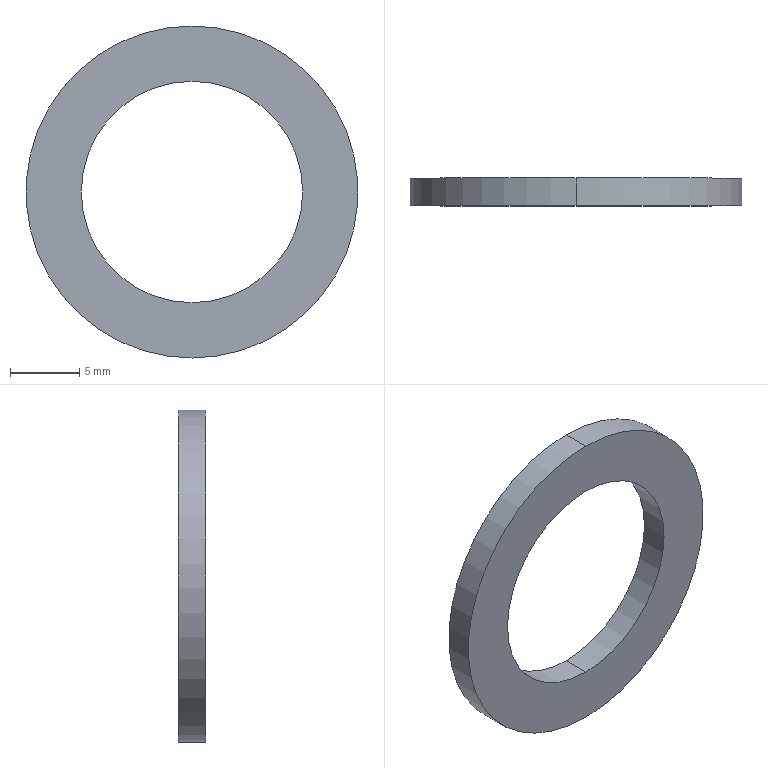Part | SolidWorks | features Extrusion 1 | 1 solid | 6 faces | box 24 x 2 x 24 mm | volume 502.655 mm3 | cylinder 4 | plane 2 | commonest cylinder face diameters 16 x2 24 x2
STEP:
#1=CARTESIAN_POINT('',(0.,2.,12.));
#2=VERTEX_POINT('',#1);
#3=CARTESIAN_POINT('',(0.,2.,-12.));
#4=VERTEX_POINT('',#3);
#5=CARTESIAN_POINT('',(0.,2.,0.));
#6=DIRECTION('',(0.,1.,0.));
#7=DIRECTION('',(0.,0.,1.));
#8=AXIS2_PLACEMENT_3D('',#5,#6,#7);
#9=CIRCLE('',#8,12.);
#10=EDGE_CURVE('',#2,#4,#9,.T.);
#11=ORIENTED_EDGE('',*,*,#10,.F.);
#12=CARTESIAN_POINT('',(0.,0.,12.));
#13=VERTEX_POINT('',#12);
#14=CARTESIAN_POINT('',(0.,2.,12.));
#15=DIRECTION('',(0.,-1.,0.));
#16=VECTOR('',#15,1000.);
#17=LINE('',#14,#16);
#18=EDGE_CURVE('',#2,#13,#17,.T.);
#19=ORIENTED_EDGE('',*,*,#18,.T.);
#20=CARTESIAN_POINT('',(0.,0.,-12.));
#21=VERTEX_POINT('',#20);
#22=CARTESIAN_POINT('',(0.,0.,0.));
#23=DIRECTION('',(0.,1.,0.));
#24=DIRECTION('',(0.,0.,1.));
#25=AXIS2_PLACEMENT_3D('',#22,#23,#24);
#26=CIRCLE('',#25,12.);
#27=EDGE_CURVE('',#13,#21,#26,.T.);
#28=ORIENTED_EDGE('',*,*,#27,.T.);
#29=CARTESIAN_POINT('',(0.,2.,-12.));
#30=DIRECTION('',(0.,-1.,0.));
#31=VECTOR('',#30,1000.);
#32=LINE('',#29,#31);
#33=EDGE_CURVE('',#4,#21,#32,.T.);
#34=ORIENTED_EDGE('',*,*,#33,.F.);
#35=EDGE_LOOP('',(#11,#19,#28,#34));
#36=FACE_OUTER_BOUND('',#35,.T.);
#37=CARTESIAN_POINT('',(0.,2.,0.));
#38=DIRECTION('',(0.,-1.,0.));
#39=DIRECTION('',(0.,0.,-1.));
#40=AXIS2_PLACEMENT_3D('',#37,#38,#39);
#41=CYLINDRICAL_SURFACE('',#40,12.);
#42=ADVANCED_FACE('',(#36),#41,.T.);
#43=CARTESIAN_POINT('',(0.,2.,-8.));
#44=VERTEX_POINT('',#43);
#45=CARTESIAN_POINT('',(0.,2.,8.));
#46=VERTEX_POINT('',#45);
#47=CARTESIAN_POINT('',(0.,2.,0.));
#48=DIRECTION('',(0.,1.,0.));
#49=DIRECTION('',(0.,0.,1.));
#50=AXIS2_PLACEMENT_3D('',#47,#48,#49);
#51=CIRCLE('',#50,8.);
#52=EDGE_CURVE('',#44,#46,#51,.T.);
#53=ORIENTED_EDGE('',*,*,#52,.T.);
#54=CARTESIAN_POINT('',(0.,0.,8.));
#55=VERTEX_POINT('',#54);
#56=CARTESIAN_POINT('',(0.,2.,8.));
#57=DIRECTION('',(0.,-1.,0.));
#58=VECTOR('',#57,1000.);
#59=LINE('',#56,#58);
#60=EDGE_CURVE('',#46,#55,#59,.T.);
#61=ORIENTED_EDGE('',*,*,#60,.T.);
#62=CARTESIAN_POINT('',(0.,0.,-8.));
#63=VERTEX_POINT('',#62);
#64=CARTESIAN_POINT('',(0.,0.,0.));
#65=DIRECTION('',(0.,1.,0.));
#66=DIRECTION('',(0.,0.,1.));
#67=AXIS2_PLACEMENT_3D('',#64,#65,#66);
#68=CIRCLE('',#67,8.);
#69=EDGE_CURVE('',#63,#55,#68,.T.);
#70=ORIENTED_EDGE('',*,*,#69,.F.);
#71=CARTESIAN_POINT('',(0.,2.,-8.));
#72=DIRECTION('',(0.,-1.,0.));
#73=VECTOR('',#72,1000.);
#74=LINE('',#71,#73);
#75=EDGE_CURVE('',#44,#63,#74,.T.);
#76=ORIENTED_EDGE('',*,*,#75,.F.);
#77=EDGE_LOOP('',(#53,#61,#70,#76));
#78=FACE_OUTER_BOUND('',#77,.T.);
#79=CARTESIAN_POINT('',(0.,2.,0.));
#80=DIRECTION('',(0.,-1.,0.));
#81=DIRECTION('',(0.,0.,-1.));
#82=AXIS2_PLACEMENT_3D('',#79,#80,#81);
#83=CYLINDRICAL_SURFACE('',#82,8.);
#84=ADVANCED_FACE('',(#78),#83,.F.);
#85=ORIENTED_EDGE('',*,*,#60,.F.);
#86=CARTESIAN_POINT('',(0.,2.,0.));
#87=DIRECTION('',(0.,1.,0.));
#88=DIRECTION('',(0.,0.,1.));
#89=AXIS2_PLACEMENT_3D('',#86,#87,#88);
#90=CIRCLE('',#89,8.);
#91=EDGE_CURVE('',#46,#44,#90,.T.);
#92=ORIENTED_EDGE('',*,*,#91,.T.);
#93=ORIENTED_EDGE('',*,*,#75,.T.);
#94=CARTESIAN_POINT('',(0.,0.,0.));
#95=DIRECTION('',(0.,1.,0.));
#96=DIRECTION('',(0.,0.,1.));
#97=AXIS2_PLACEMENT_3D('',#94,#95,#96);
#98=CIRCLE('',#97,8.);
#99=EDGE_CURVE('',#55,#63,#98,.T.);
#100=ORIENTED_EDGE('',*,*,#99,.F.);
#101=EDGE_LOOP('',(#85,#92,#93,#100));
#102=FACE_OUTER_BOUND('',#101,.T.);
#103=CARTESIAN_POINT('',(0.,2.,0.));
#104=DIRECTION('',(0.,-1.,0.));
#105=DIRECTION('',(0.,0.,-1.));
#106=AXIS2_PLACEMENT_3D('',#103,#104,#105);
#107=CYLINDRICAL_SURFACE('',#106,8.);
#108=ADVANCED_FACE('',(#102),#107,.F.);
#109=ORIENTED_EDGE('',*,*,#18,.F.);
#110=CARTESIAN_POINT('',(0.,2.,0.));
#111=DIRECTION('',(0.,1.,0.));
#112=DIRECTION('',(0.,0.,1.));
#113=AXIS2_PLACEMENT_3D('',#110,#111,#112);
#114=CIRCLE('',#113,12.);
#115=EDGE_CURVE('',#4,#2,#114,.T.);
#116=ORIENTED_EDGE('',*,*,#115,.F.);
#117=ORIENTED_EDGE('',*,*,#33,.T.);
#118=CARTESIAN_POINT('',(0.,0.,0.));
#119=DIRECTION('',(0.,1.,0.));
#120=DIRECTION('',(0.,0.,1.));
#121=AXIS2_PLACEMENT_3D('',#118,#119,#120);
#122=CIRCLE('',#121,12.);
#123=EDGE_CURVE('',#21,#13,#122,.T.);
#124=ORIENTED_EDGE('',*,*,#123,.T.);
#125=EDGE_LOOP('',(#109,#116,#117,#124));
#126=FACE_OUTER_BOUND('',#125,.T.);
#127=CARTESIAN_POINT('',(0.,2.,0.));
#128=DIRECTION('',(0.,-1.,0.));
#129=DIRECTION('',(0.,0.,-1.));
#130=AXIS2_PLACEMENT_3D('',#127,#128,#129);
#131=CYLINDRICAL_SURFACE('',#130,12.);
#132=ADVANCED_FACE('',(#126),#131,.T.);
#133=ORIENTED_EDGE('',*,*,#52,.F.);
#134=ORIENTED_EDGE('',*,*,#91,.F.);
#135=EDGE_LOOP('',(#133,#134));
#136=FACE_BOUND('',#135,.T.);
#137=ORIENTED_EDGE('',*,*,#115,.T.);
#138=ORIENTED_EDGE('',*,*,#10,.T.);
#139=EDGE_LOOP('',(#137,#138));
#140=FACE_OUTER_BOUND('',#139,.T.);
#141=CARTESIAN_POINT('',(0.,2.,0.));
#142=DIRECTION('',(0.,1.,0.));
#143=DIRECTION('',(0.,0.,1.));
#144=AXIS2_PLACEMENT_3D('',#141,#142,#143);
#145=PLANE('',#144);
#146=ADVANCED_FACE('',(#136,#140),#145,.T.);
#147=ORIENTED_EDGE('',*,*,#69,.T.);
#148=ORIENTED_EDGE('',*,*,#99,.T.);
#149=EDGE_LOOP('',(#147,#148));
#150=FACE_BOUND('',#149,.T.);
#151=ORIENTED_EDGE('',*,*,#123,.F.);
#152=ORIENTED_EDGE('',*,*,#27,.F.);
#153=EDGE_LOOP('',(#151,#152));
#154=FACE_OUTER_BOUND('',#153,.T.);
#155=CARTESIAN_POINT('',(0.,0.,0.));
#156=DIRECTION('',(0.,1.,0.));
#157=DIRECTION('',(0.,0.,1.));
#158=AXIS2_PLACEMENT_3D('',#155,#156,#157);
#159=PLANE('',#158);
#160=ADVANCED_FACE('',(#150,#154),#159,.F.);
#161=CLOSED_SHELL('',(#42,#84,#108,#132,#146,#160));
#162=MANIFOLD_SOLID_BREP('',#161);
#163=CARTESIAN_POINT('',(0.,0.,0.));
#164=DIRECTION('',(0.,0.,1.));
#165=DIRECTION('',(1.,0.,0.));
#166=AXIS2_PLACEMENT_3D('',#163,#164,#165);
#167=(LENGTH_UNIT()NAMED_UNIT(*)SI_UNIT(.MILLI.,.METRE.));
#168=UNCERTAINTY_MEASURE_WITH_UNIT(LENGTH_MEASURE(0.00001),#167,'','');
#169=(NAMED_UNIT(*)PLANE_ANGLE_UNIT()SI_UNIT($,.RADIAN.));
#170=(NAMED_UNIT(*)SI_UNIT($,.STERADIAN.)SOLID_ANGLE_UNIT());
#171=(GEOMETRIC_REPRESENTATION_CONTEXT(3)GLOBAL_UNCERTAINTY_ASSIGNED_CONTEXT((#168))GLOBAL_UNIT_ASSIGNED_CONTEXT((#167,#169,#170))REPRESENTATION_CONTEXT('',''));
#172=ADVANCED_BREP_SHAPE_REPRESENTATION('',(#162,#166),#171);